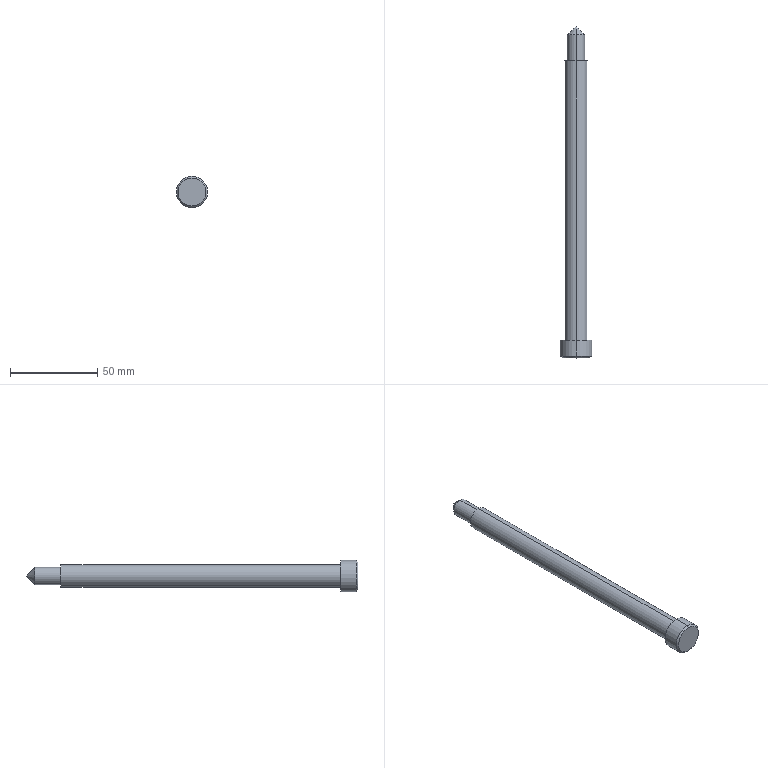Part | STEP file | 1 solid | 13 faces | box 18 x 190 x 18 mm | volume 25064 mm3 | cylinder 6 | cone 4 | plane 3 | commonest cylinder face diameters 10 x2 13 x2 18 x2
STEP:
#1=CARTESIAN_POINT('',(0.,0.,0.));
#2=DIRECTION('',(0.,0.,1.));
#3=DIRECTION('',(1.,0.,0.));
#4=AXIS2_PLACEMENT_3D('',#1,#2,#3);
#5=CARTESIAN_POINT('',(-72.862,-218.5,40.53));
#6=VERTEX_POINT('',#5);
#7=CARTESIAN_POINT('',(-72.862,-218.5,56.53));
#8=VERTEX_POINT('',#7);
#9=CARTESIAN_POINT('',(-72.862,-218.5,48.53));
#10=DIRECTION('',(0.,-1.,0.));
#11=DIRECTION('',(0.,0.,1.));
#12=AXIS2_PLACEMENT_3D('',#9,#10,#11);
#13=CIRCLE('',#12,8.);
#14=CARTESIAN_POINT('',(-72.862,-217.5,48.53));
#15=DIRECTION('',(0.,1.,0.));
#16=DIRECTION('',(0.,0.,1.));
#17=AXIS2_PLACEMENT_3D('',#14,#15,#16);
#18=CONICAL_SURFACE('',#17,9.,0.7854);
#19=CARTESIAN_POINT('',(6.283,-1.));
#20=DIRECTION('',(-1.,0.));
#21=VECTOR('',#20,1.);
#22=LINE('',#19,#21);
#23=(GEOMETRIC_REPRESENTATION_CONTEXT(2)PARAMETRIC_REPRESENTATION_CONTEXT()REPRESENTATION_CONTEXT('',''));
#24=DEFINITIONAL_REPRESENTATION('',(#22),#23);
#25=PCURVE('',#18,#24);
#26=CARTESIAN_POINT('',(-72.862,-218.5,48.53));
#27=DIRECTION('',(0.,1.,0.));
#28=DIRECTION('',(0.,0.,1.));
#29=AXIS2_PLACEMENT_3D('',#26,#27,#28);
#30=PLANE('',#29);
#31=CARTESIAN_POINT('',(8.,0.));
#32=CARTESIAN_POINT('',(8.,-13.856));
#33=CARTESIAN_POINT('',(-4.,-6.928));
#34=CARTESIAN_POINT('',(-16.,0.));
#35=CARTESIAN_POINT('',(-4.,6.928));
#36=CARTESIAN_POINT('',(8.,13.856));
#37=CARTESIAN_POINT('',(8.,0.));
#38=(BOUNDED_CURVE()B_SPLINE_CURVE(2,(#31,#32,#33,#34,#35,#36,#37),.UNSPECIFIED.,.T.,.F.)B_SPLINE_CURVE_WITH_KNOTS((1,2,2,2,2,1),(-2.094,0.,2.094,4.189,6.283,8.378),.UNSPECIFIED.)CURVE()GEOMETRIC_REPRESENTATION_ITEM()RATIONAL_B_SPLINE_CURVE((1.,0.5,1.,0.5,1.,0.5,1.))REPRESENTATION_ITEM(''));
#39=(GEOMETRIC_REPRESENTATION_CONTEXT(2)PARAMETRIC_REPRESENTATION_CONTEXT()REPRESENTATION_CONTEXT('',''));
#40=DEFINITIONAL_REPRESENTATION('',(#38),#39);
#41=PCURVE('',#30,#40);
#42=SURFACE_CURVE('',#13,(#25,#41),.PCURVE_S1.);
#43=EDGE_CURVE('',#6,#8,#42,.T.);
#44=ORIENTED_EDGE('',*,*,#43,.F.);
#45=CARTESIAN_POINT('',(-72.862,-217.5,39.53));
#46=VERTEX_POINT('',#45);
#47=CARTESIAN_POINT('',(-72.862,-217.5,39.53));
#48=DIRECTION('',(0.,0.7071,-0.7071));
#49=VECTOR('',#48,1.);
#50=LINE('',#47,#49);
#51=CARTESIAN_POINT('',(3.142,0.));
#52=DIRECTION('',(0.,1.));
#53=VECTOR('',#52,1.);
#54=LINE('',#51,#53);
#55=(GEOMETRIC_REPRESENTATION_CONTEXT(2)PARAMETRIC_REPRESENTATION_CONTEXT()REPRESENTATION_CONTEXT('',''));
#56=DEFINITIONAL_REPRESENTATION('',(#54),#55);
#57=PCURVE('',#18,#56);
#58=CARTESIAN_POINT('',(-72.862,-217.5,48.53));
#59=DIRECTION('',(0.,1.,0.));
#60=DIRECTION('',(0.,0.,1.));
#61=AXIS2_PLACEMENT_3D('',#58,#59,#60);
#62=CONICAL_SURFACE('',#61,9.,0.7854);
#63=CARTESIAN_POINT('',(3.142,0.));
#64=DIRECTION('',(0.,1.));
#65=VECTOR('',#64,1.);
#66=LINE('',#63,#65);
#67=(GEOMETRIC_REPRESENTATION_CONTEXT(2)PARAMETRIC_REPRESENTATION_CONTEXT()REPRESENTATION_CONTEXT('',''));
#68=DEFINITIONAL_REPRESENTATION('',(#66),#67);
#69=PCURVE('',#62,#68);
#70=SURFACE_CURVE('',#50,(#57,#69),.PCURVE_S1.);
#71=EDGE_CURVE('',#6,#46,#70,.T.);
#72=ORIENTED_EDGE('',*,*,#71,.T.);
#73=CARTESIAN_POINT('',(-72.862,-217.5,57.53));
#74=VERTEX_POINT('',#73);
#75=CARTESIAN_POINT('',(-72.862,-217.5,48.53));
#76=DIRECTION('',(0.,1.,0.));
#77=DIRECTION('',(0.,0.,1.));
#78=AXIS2_PLACEMENT_3D('',#75,#76,#77);
#79=CIRCLE('',#78,9.);
#80=CARTESIAN_POINT('',(0.,0.));
#81=DIRECTION('',(1.,0.));
#82=VECTOR('',#81,1.);
#83=LINE('',#80,#82);
#84=(GEOMETRIC_REPRESENTATION_CONTEXT(2)PARAMETRIC_REPRESENTATION_CONTEXT()REPRESENTATION_CONTEXT('',''));
#85=DEFINITIONAL_REPRESENTATION('',(#83),#84);
#86=PCURVE('',#18,#85);
#87=CARTESIAN_POINT('',(-72.862,-220.,48.53));
#88=DIRECTION('',(0.,1.,0.));
#89=DIRECTION('',(0.,0.,1.));
#90=AXIS2_PLACEMENT_3D('',#87,#88,#89);
#91=CYLINDRICAL_SURFACE('',#90,9.);
#92=CARTESIAN_POINT('',(0.,2.5));
#93=DIRECTION('',(1.,0.));
#94=VECTOR('',#93,1.);
#95=LINE('',#92,#94);
#96=(GEOMETRIC_REPRESENTATION_CONTEXT(2)PARAMETRIC_REPRESENTATION_CONTEXT()REPRESENTATION_CONTEXT('',''));
#97=DEFINITIONAL_REPRESENTATION('',(#95),#96);
#98=PCURVE('',#91,#97);
#99=SURFACE_CURVE('',#79,(#86,#98),.PCURVE_S1.);
#100=EDGE_CURVE('',#74,#46,#99,.T.);
#101=ORIENTED_EDGE('',*,*,#100,.F.);
#102=CARTESIAN_POINT('',(-72.862,-217.5,57.53));
#103=DIRECTION('',(0.,0.7071,0.7071));
#104=VECTOR('',#103,1.);
#105=LINE('',#102,#104);
#106=CARTESIAN_POINT('',(0.,0.));
#107=DIRECTION('',(0.,1.));
#108=VECTOR('',#107,1.);
#109=LINE('',#106,#108);
#110=(GEOMETRIC_REPRESENTATION_CONTEXT(2)PARAMETRIC_REPRESENTATION_CONTEXT()REPRESENTATION_CONTEXT('',''));
#111=DEFINITIONAL_REPRESENTATION('',(#109),#110);
#112=PCURVE('',#18,#111);
#113=CARTESIAN_POINT('',(6.283,0.));
#114=DIRECTION('',(0.,1.));
#115=VECTOR('',#114,1.);
#116=LINE('',#113,#115);
#117=(GEOMETRIC_REPRESENTATION_CONTEXT(2)PARAMETRIC_REPRESENTATION_CONTEXT()REPRESENTATION_CONTEXT('',''));
#118=DEFINITIONAL_REPRESENTATION('',(#116),#117);
#119=PCURVE('',#62,#118);
#120=SURFACE_CURVE('',#105,(#112,#119),.PCURVE_S1.);
#121=EDGE_CURVE('',#8,#74,#120,.T.);
#122=ORIENTED_EDGE('',*,*,#121,.F.);
#123=EDGE_LOOP('',(#44,#72,#101,#122));
#124=FACE_BOUND('',#123,.T.);
#125=ADVANCED_FACE('',(#124),#18,.T.);
#126=CARTESIAN_POINT('',(-72.862,-28.5,48.53));
#127=VERTEX_POINT('',#126);
#128=CARTESIAN_POINT('',(-72.862,-33.5,43.53));
#129=VERTEX_POINT('',#128);
#130=CARTESIAN_POINT('',(-72.862,-33.5,43.53));
#131=DIRECTION('',(0.,-0.7071,-0.7071));
#132=VECTOR('',#131,1.);
#133=LINE('',#130,#132);
#134=CARTESIAN_POINT('',(-72.862,-33.5,48.53));
#135=DIRECTION('',(0.,-1.,0.));
#136=DIRECTION('',(0.,0.,-1.));
#137=AXIS2_PLACEMENT_3D('',#134,#135,#136);
#138=CONICAL_SURFACE('',#137,5.,0.7854);
#139=CARTESIAN_POINT('',(0.,0.));
#140=DIRECTION('',(0.,1.));
#141=VECTOR('',#140,1.);
#142=LINE('',#139,#141);
#143=(GEOMETRIC_REPRESENTATION_CONTEXT(2)PARAMETRIC_REPRESENTATION_CONTEXT()REPRESENTATION_CONTEXT('',''));
#144=DEFINITIONAL_REPRESENTATION('',(#142),#143);
#145=PCURVE('',#138,#144);
#146=CARTESIAN_POINT('',(-72.862,-33.5,48.53));
#147=DIRECTION('',(0.,-1.,0.));
#148=DIRECTION('',(0.,0.,-1.));
#149=AXIS2_PLACEMENT_3D('',#146,#147,#148);
#150=CONICAL_SURFACE('',#149,5.,0.7854);
#151=CARTESIAN_POINT('',(6.283,0.));
#152=DIRECTION('',(0.,1.));
#153=VECTOR('',#152,1.);
#154=LINE('',#151,#153);
#155=(GEOMETRIC_REPRESENTATION_CONTEXT(2)PARAMETRIC_REPRESENTATION_CONTEXT()REPRESENTATION_CONTEXT('',''));
#156=DEFINITIONAL_REPRESENTATION('',(#154),#155);
#157=PCURVE('',#150,#156);
#158=SURFACE_CURVE('',#133,(#145,#157),.PCURVE_S1.);
#159=EDGE_CURVE('',#127,#129,#158,.T.);
#160=ORIENTED_EDGE('',*,*,#159,.F.);
#161=CARTESIAN_POINT('',(-72.862,-33.5,53.53));
#162=VERTEX_POINT('',#161);
#163=CARTESIAN_POINT('',(-72.862,-33.5,53.53));
#164=DIRECTION('',(0.,-0.7071,0.7071));
#165=VECTOR('',#164,1.);
#166=LINE('',#163,#165);
#167=CARTESIAN_POINT('',(3.142,-5.));
#168=CARTESIAN_POINT('',(3.142,-4.924));
#169=CARTESIAN_POINT('',(3.142,-4.773));
#170=CARTESIAN_POINT('',(3.142,-4.545));
#171=CARTESIAN_POINT('',(3.142,-4.318));
#172=CARTESIAN_POINT('',(3.142,-4.091));
#173=CARTESIAN_POINT('',(3.142,-3.864));
#174=CARTESIAN_POINT('',(3.142,-3.636));
#175=CARTESIAN_POINT('',(3.142,-3.409));
#176=CARTESIAN_POINT('',(3.142,-3.182));
#177=CARTESIAN_POINT('',(3.142,-2.955));
#178=CARTESIAN_POINT('',(3.142,-2.727));
#179=CARTESIAN_POINT('',(3.142,-2.5));
#180=CARTESIAN_POINT('',(3.142,-2.273));
#181=CARTESIAN_POINT('',(3.142,-2.045));
#182=CARTESIAN_POINT('',(3.142,-1.818));
#183=CARTESIAN_POINT('',(3.142,-1.591));
#184=CARTESIAN_POINT('',(3.142,-1.364));
#185=CARTESIAN_POINT('',(3.142,-1.136));
#186=CARTESIAN_POINT('',(3.142,-0.9091));
#187=CARTESIAN_POINT('',(3.142,-0.6818));
#188=CARTESIAN_POINT('',(3.142,-0.4545));
#189=CARTESIAN_POINT('',(3.142,-0.2273));
#190=CARTESIAN_POINT('',(3.142,-0.07576));
#191=CARTESIAN_POINT('',(3.142,0.));
#192=B_SPLINE_CURVE_WITH_KNOTS('',3,(#167,#168,#169,#170,#171,#172,#173,#174,#175,#176,#177,#178,#179,#180,#181,#182,#183,#184,#185,#186,#187,#188,#189,#190,#191),.UNSPECIFIED.,.F.,.F.,(4,1,1,1,1,1,1,1,1,1,1,1,1,1,1,1,1,1,1,1,1,1,4),(-7.071,-6.75,-6.428,-6.107,-5.785,-5.464,-5.143,-4.821,-4.5,-4.178,-3.857,-3.536,-3.214,-2.893,-2.571,-2.25,-1.928,-1.607,-1.286,-0.9642,-0.6428,-0.3214,0.),.QUASI_UNIFORM_KNOTS.);
#193=(GEOMETRIC_REPRESENTATION_CONTEXT(2)PARAMETRIC_REPRESENTATION_CONTEXT()REPRESENTATION_CONTEXT('',''));
#194=DEFINITIONAL_REPRESENTATION('',(#192),#193);
#195=PCURVE('',#138,#194);
#196=CARTESIAN_POINT('',(3.142,-5.));
#197=CARTESIAN_POINT('',(3.142,-4.924));
#198=CARTESIAN_POINT('',(3.142,-4.773));
#199=CARTESIAN_POINT('',(3.142,-4.545));
#200=CARTESIAN_POINT('',(3.142,-4.318));
#201=CARTESIAN_POINT('',(3.142,-4.091));
#202=CARTESIAN_POINT('',(3.142,-3.864));
#203=CARTESIAN_POINT('',(3.142,-3.636));
#204=CARTESIAN_POINT('',(3.142,-3.409));
#205=CARTESIAN_POINT('',(3.142,-3.182));
#206=CARTESIAN_POINT('',(3.142,-2.955));
#207=CARTESIAN_POINT('',(3.142,-2.727));
#208=CARTESIAN_POINT('',(3.142,-2.5));
#209=CARTESIAN_POINT('',(3.142,-2.273));
#210=CARTESIAN_POINT('',(3.142,-2.045));
#211=CARTESIAN_POINT('',(3.142,-1.818));
#212=CARTESIAN_POINT('',(3.142,-1.591));
#213=CARTESIAN_POINT('',(3.142,-1.364));
#214=CARTESIAN_POINT('',(3.142,-1.136));
#215=CARTESIAN_POINT('',(3.142,-0.9091));
#216=CARTESIAN_POINT('',(3.142,-0.6818));
#217=CARTESIAN_POINT('',(3.142,-0.4545));
#218=CARTESIAN_POINT('',(3.142,-0.2273));
#219=CARTESIAN_POINT('',(3.142,-0.07576));
#220=CARTESIAN_POINT('',(3.142,0.));
#221=B_SPLINE_CURVE_WITH_KNOTS('',3,(#196,#197,#198,#199,#200,#201,#202,#203,#204,#205,#206,#207,#208,#209,#210,#211,#212,#213,#214,#215,#216,#217,#218,#219,#220),.UNSPECIFIED.,.F.,.F.,(4,1,1,1,1,1,1,1,1,1,1,1,1,1,1,1,1,1,1,1,1,1,4),(-7.071,-6.75,-6.428,-6.107,-5.785,-5.464,-5.143,-4.821,-4.5,-4.178,-3.857,-3.536,-3.214,-2.893,-2.571,-2.25,-1.928,-1.607,-1.286,-0.9642,-0.6428,-0.3214,0.),.QUASI_UNIFORM_KNOTS.);
#222=(GEOMETRIC_REPRESENTATION_CONTEXT(2)PARAMETRIC_REPRESENTATION_CONTEXT()REPRESENTATION_CONTEXT('',''));
#223=DEFINITIONAL_REPRESENTATION('',(#221),#222);
#224=PCURVE('',#150,#223);
#225=SURFACE_CURVE('',#166,(#195,#224),.PCURVE_S1.);
#226=EDGE_CURVE('',#127,#162,#225,.T.);
#227=ORIENTED_EDGE('',*,*,#226,.T.);
#228=CARTESIAN_POINT('',(-72.862,-33.5,48.53));
#229=DIRECTION('',(0.,-1.,0.));
#230=DIRECTION('',(0.,0.,1.));
#231=AXIS2_PLACEMENT_3D('',#228,#229,#230);
#232=CIRCLE('',#231,5.);
#233=CARTESIAN_POINT('',(-3.142,0.));
#234=DIRECTION('',(1.,0.));
#235=VECTOR('',#234,1.);
#236=LINE('',#233,#235);
#237=(GEOMETRIC_REPRESENTATION_CONTEXT(2)PARAMETRIC_REPRESENTATION_CONTEXT()REPRESENTATION_CONTEXT('',''));
#238=DEFINITIONAL_REPRESENTATION('',(#236),#237);
#239=PCURVE('',#138,#238);
#240=CARTESIAN_POINT('',(-72.862,-48.5,48.53));
#241=DIRECTION('',(0.,1.,0.));
#242=DIRECTION('',(0.,0.,1.));
#243=AXIS2_PLACEMENT_3D('',#240,#241,#242);
#244=CYLINDRICAL_SURFACE('',#243,5.);
#245=CARTESIAN_POINT('',(6.283,15.));
#246=DIRECTION('',(-1.,0.));
#247=VECTOR('',#246,1.);
#248=LINE('',#245,#247);
#249=(GEOMETRIC_REPRESENTATION_CONTEXT(2)PARAMETRIC_REPRESENTATION_CONTEXT()REPRESENTATION_CONTEXT('',''));
#250=DEFINITIONAL_REPRESENTATION('',(#248),#249);
#251=PCURVE('',#244,#250);
#252=SURFACE_CURVE('',#232,(#239,#251),.PCURVE_S1.);
#253=EDGE_CURVE('',#129,#162,#252,.T.);
#254=ORIENTED_EDGE('',*,*,#253,.F.);
#255=EDGE_LOOP('',(#160,#227,#254));
#256=FACE_BOUND('',#255,.T.);
#257=ADVANCED_FACE('',(#256),#138,.T.);
#258=CARTESIAN_POINT('',(-72.862,-48.5,53.53));
#259=VERTEX_POINT('',#258);
#260=CARTESIAN_POINT('',(-72.862,-48.5,43.53));
#261=VERTEX_POINT('',#260);
#262=CARTESIAN_POINT('',(-72.862,-48.5,48.53));
#263=DIRECTION('',(0.,1.,0.));
#264=DIRECTION('',(0.,0.,1.));
#265=AXIS2_PLACEMENT_3D('',#262,#263,#264);
#266=CIRCLE('',#265,5.);
#267=CARTESIAN_POINT('',(0.,0.));
#268=DIRECTION('',(1.,0.));
#269=VECTOR('',#268,1.);
#270=LINE('',#267,#269);
#271=(GEOMETRIC_REPRESENTATION_CONTEXT(2)PARAMETRIC_REPRESENTATION_CONTEXT()REPRESENTATION_CONTEXT('',''));
#272=DEFINITIONAL_REPRESENTATION('',(#270),#271);
#273=PCURVE('',#244,#272);
#274=CARTESIAN_POINT('',(-72.862,-48.5,48.53));
#275=DIRECTION('',(0.,1.,0.));
#276=DIRECTION('',(0.,0.,1.));
#277=AXIS2_PLACEMENT_3D('',#274,#275,#276);
#278=PLANE('',#277);
#279=CARTESIAN_POINT('',(0.,0.));
#280=DIRECTION('',(1.,0.));
#281=AXIS2_PLACEMENT_2D('',#279,#280);
#282=CIRCLE('',#281,5.);
#283=(GEOMETRIC_REPRESENTATION_CONTEXT(2)PARAMETRIC_REPRESENTATION_CONTEXT()REPRESENTATION_CONTEXT('',''));
#284=DEFINITIONAL_REPRESENTATION('',(#282),#283);
#285=PCURVE('',#278,#284);
#286=SURFACE_CURVE('',#266,(#273,#285),.PCURVE_S1.);
#287=EDGE_CURVE('',#259,#261,#286,.T.);
#288=ORIENTED_EDGE('',*,*,#287,.T.);
#289=CARTESIAN_POINT('',(-72.862,-48.5,43.53));
#290=DIRECTION('',(0.,1.,0.));
#291=VECTOR('',#290,1.);
#292=LINE('',#289,#291);
#293=CARTESIAN_POINT('',(3.142,0.));
#294=DIRECTION('',(0.,1.));
#295=VECTOR('',#294,1.);
#296=LINE('',#293,#295);
#297=(GEOMETRIC_REPRESENTATION_CONTEXT(2)PARAMETRIC_REPRESENTATION_CONTEXT()REPRESENTATION_CONTEXT('',''));
#298=DEFINITIONAL_REPRESENTATION('',(#296),#297);
#299=PCURVE('',#244,#298);
#300=CARTESIAN_POINT('',(-72.862,-48.5,48.53));
#301=DIRECTION('',(0.,1.,0.));
#302=DIRECTION('',(0.,0.,1.));
#303=AXIS2_PLACEMENT_3D('',#300,#301,#302);
#304=CYLINDRICAL_SURFACE('',#303,5.);
#305=CARTESIAN_POINT('',(3.142,0.));
#306=DIRECTION('',(0.,1.));
#307=VECTOR('',#306,1.);
#308=LINE('',#305,#307);
#309=(GEOMETRIC_REPRESENTATION_CONTEXT(2)PARAMETRIC_REPRESENTATION_CONTEXT()REPRESENTATION_CONTEXT('',''));
#310=DEFINITIONAL_REPRESENTATION('',(#308),#309);
#311=PCURVE('',#304,#310);
#312=SURFACE_CURVE('',#292,(#299,#311),.PCURVE_S1.);
#313=EDGE_CURVE('',#261,#129,#312,.T.);
#314=ORIENTED_EDGE('',*,*,#313,.T.);
#315=ORIENTED_EDGE('',*,*,#253,.T.);
#316=CARTESIAN_POINT('',(-72.862,-48.5,53.53));
#317=DIRECTION('',(0.,1.,0.));
#318=VECTOR('',#317,1.);
#319=LINE('',#316,#318);
#320=CARTESIAN_POINT('',(0.,0.));
#321=DIRECTION('',(0.,1.));
#322=VECTOR('',#321,1.);
#323=LINE('',#320,#322);
#324=(GEOMETRIC_REPRESENTATION_CONTEXT(2)PARAMETRIC_REPRESENTATION_CONTEXT()REPRESENTATION_CONTEXT('',''));
#325=DEFINITIONAL_REPRESENTATION('',(#323),#324);
#326=PCURVE('',#244,#325);
#327=CARTESIAN_POINT('',(6.283,0.));
#328=DIRECTION('',(0.,1.));
#329=VECTOR('',#328,1.);
#330=LINE('',#327,#329);
#331=(GEOMETRIC_REPRESENTATION_CONTEXT(2)PARAMETRIC_REPRESENTATION_CONTEXT()REPRESENTATION_CONTEXT('',''));
#332=DEFINITIONAL_REPRESENTATION('',(#330),#331);
#333=PCURVE('',#304,#332);
#334=SURFACE_CURVE('',#319,(#326,#333),.PCURVE_S1.);
#335=EDGE_CURVE('',#259,#162,#334,.T.);
#336=ORIENTED_EDGE('',*,*,#335,.F.);
#337=EDGE_LOOP('',(#288,#314,#315,#336));
#338=FACE_BOUND('',#337,.T.);
#339=ADVANCED_FACE('',(#338),#244,.T.);
#340=CARTESIAN_POINT('',(-72.862,-208.5,55.03));
#341=VERTEX_POINT('',#340);
#342=CARTESIAN_POINT('',(-72.862,-208.5,42.03));
#343=VERTEX_POINT('',#342);
#344=CARTESIAN_POINT('',(-72.862,-208.5,48.53));
#345=DIRECTION('',(0.,1.,0.));
#346=DIRECTION('',(0.,0.,-1.));
#347=AXIS2_PLACEMENT_3D('',#344,#345,#346);
#348=CIRCLE('',#347,6.5);
#349=CARTESIAN_POINT('',(-72.862,-220.,48.53));
#350=DIRECTION('',(0.,1.,0.));
#351=DIRECTION('',(0.,0.,1.));
#352=AXIS2_PLACEMENT_3D('',#349,#350,#351);
#353=CYLINDRICAL_SURFACE('',#352,6.5);
#354=CARTESIAN_POINT('',(-3.142,11.5));
#355=DIRECTION('',(1.,0.));
#356=VECTOR('',#355,1.);
#357=LINE('',#354,#356);
#358=(GEOMETRIC_REPRESENTATION_CONTEXT(2)PARAMETRIC_REPRESENTATION_CONTEXT()REPRESENTATION_CONTEXT('',''));
#359=DEFINITIONAL_REPRESENTATION('',(#357),#358);
#360=PCURVE('',#353,#359);
#361=CARTESIAN_POINT('',(-72.862,-208.5,48.53));
#362=DIRECTION('',(0.,-1.,0.));
#363=DIRECTION('',(0.,0.,-1.));
#364=AXIS2_PLACEMENT_3D('',#361,#362,#363);
#365=PLANE('',#364);
#366=CARTESIAN_POINT('',(6.5,0.));
#367=CARTESIAN_POINT('',(6.5,-11.258));
#368=CARTESIAN_POINT('',(-3.25,-5.629));
#369=CARTESIAN_POINT('',(-13.,0.));
#370=CARTESIAN_POINT('',(-3.25,5.629));
#371=CARTESIAN_POINT('',(6.5,11.258));
#372=CARTESIAN_POINT('',(6.5,0.));
#373=(BOUNDED_CURVE()B_SPLINE_CURVE(2,(#366,#367,#368,#369,#370,#371,#372),.UNSPECIFIED.,.T.,.F.)B_SPLINE_CURVE_WITH_KNOTS((1,2,2,2,2,1),(-2.094,0.,2.094,4.189,6.283,8.378),.UNSPECIFIED.)CURVE()GEOMETRIC_REPRESENTATION_ITEM()RATIONAL_B_SPLINE_CURVE((1.,0.5,1.,0.5,1.,0.5,1.))REPRESENTATION_ITEM(''));
#374=(GEOMETRIC_REPRESENTATION_CONTEXT(2)PARAMETRIC_REPRESENTATION_CONTEXT()REPRESENTATION_CONTEXT('',''));
#375=DEFINITIONAL_REPRESENTATION('',(#373),#374);
#376=PCURVE('',#365,#375);
#377=SURFACE_CURVE('',#348,(#360,#376),.PCURVE_S1.);
#378=EDGE_CURVE('',#341,#343,#377,.T.);
#379=ORIENTED_EDGE('',*,*,#378,.T.);
#380=CARTESIAN_POINT('',(-72.862,-48.5,42.03));
#381=VERTEX_POINT('',#380);
#382=CARTESIAN_POINT('',(-72.862,-220.,42.03));
#383=DIRECTION('',(0.,1.,0.));
#384=VECTOR('',#383,1.);
#385=LINE('',#382,#384);
#386=CARTESIAN_POINT('',(3.142,0.));
#387=DIRECTION('',(0.,1.));
#388=VECTOR('',#387,1.);
#389=LINE('',#386,#388);
#390=(GEOMETRIC_REPRESENTATION_CONTEXT(2)PARAMETRIC_REPRESENTATION_CONTEXT()REPRESENTATION_CONTEXT('',''));
#391=DEFINITIONAL_REPRESENTATION('',(#389),#390);
#392=PCURVE('',#353,#391);
#393=CARTESIAN_POINT('',(-72.862,-220.,48.53));
#394=DIRECTION('',(0.,1.,0.));
#395=DIRECTION('',(0.,0.,1.));
#396=AXIS2_PLACEMENT_3D('',#393,#394,#395);
#397=CYLINDRICAL_SURFACE('',#396,6.5);
#398=CARTESIAN_POINT('',(3.142,0.));
#399=DIRECTION('',(0.,1.));
#400=VECTOR('',#399,1.);
#401=LINE('',#398,#400);
#402=(GEOMETRIC_REPRESENTATION_CONTEXT(2)PARAMETRIC_REPRESENTATION_CONTEXT()REPRESENTATION_CONTEXT('',''));
#403=DEFINITIONAL_REPRESENTATION('',(#401),#402);
#404=PCURVE('',#397,#403);
#405=SURFACE_CURVE('',#385,(#392,#404),.PCURVE_S1.);
#406=EDGE_CURVE('',#343,#381,#405,.T.);
#407=ORIENTED_EDGE('',*,*,#406,.T.);
#408=CARTESIAN_POINT('',(-72.862,-48.5,55.03));
#409=VERTEX_POINT('',#408);
#410=CARTESIAN_POINT('',(-72.862,-48.5,48.53));
#411=DIRECTION('',(0.,1.,0.));
#412=DIRECTION('',(0.,0.,1.));
#413=AXIS2_PLACEMENT_3D('',#410,#411,#412);
#414=CIRCLE('',#413,6.5);
#415=CARTESIAN_POINT('',(0.,171.5));
#416=DIRECTION('',(1.,0.));
#417=VECTOR('',#416,1.);
#418=LINE('',#415,#417);
#419=(GEOMETRIC_REPRESENTATION_CONTEXT(2)PARAMETRIC_REPRESENTATION_CONTEXT()REPRESENTATION_CONTEXT('',''));
#420=DEFINITIONAL_REPRESENTATION('',(#418),#419);
#421=PCURVE('',#353,#420);
#422=CARTESIAN_POINT('',(0.,0.));
#423=DIRECTION('',(1.,0.));
#424=AXIS2_PLACEMENT_2D('',#422,#423);
#425=CIRCLE('',#424,6.5);
#426=(GEOMETRIC_REPRESENTATION_CONTEXT(2)PARAMETRIC_REPRESENTATION_CONTEXT()REPRESENTATION_CONTEXT('',''));
#427=DEFINITIONAL_REPRESENTATION('',(#425),#426);
#428=PCURVE('',#278,#427);
#429=SURFACE_CURVE('',#414,(#421,#428),.PCURVE_S1.);
#430=EDGE_CURVE('',#409,#381,#429,.T.);
#431=ORIENTED_EDGE('',*,*,#430,.F.);
#432=CARTESIAN_POINT('',(-72.862,-220.,55.03));
#433=DIRECTION('',(0.,1.,0.));
#434=VECTOR('',#433,1.);
#435=LINE('',#432,#434);
#436=CARTESIAN_POINT('',(0.,0.));
#437=DIRECTION('',(0.,1.));
#438=VECTOR('',#437,1.);
#439=LINE('',#436,#438);
#440=(GEOMETRIC_REPRESENTATION_CONTEXT(2)PARAMETRIC_REPRESENTATION_CONTEXT()REPRESENTATION_CONTEXT('',''));
#441=DEFINITIONAL_REPRESENTATION('',(#439),#440);
#442=PCURVE('',#353,#441);
#443=CARTESIAN_POINT('',(6.283,0.));
#444=DIRECTION('',(0.,1.));
#445=VECTOR('',#444,1.);
#446=LINE('',#443,#445);
#447=(GEOMETRIC_REPRESENTATION_CONTEXT(2)PARAMETRIC_REPRESENTATION_CONTEXT()REPRESENTATION_CONTEXT('',''));
#448=DEFINITIONAL_REPRESENTATION('',(#446),#447);
#449=PCURVE('',#397,#448);
#450=SURFACE_CURVE('',#435,(#442,#449),.PCURVE_S1.);
#451=EDGE_CURVE('',#341,#409,#450,.T.);
#452=ORIENTED_EDGE('',*,*,#451,.F.);
#453=EDGE_LOOP('',(#379,#407,#431,#452));
#454=FACE_BOUND('',#453,.T.);
#455=ADVANCED_FACE('',(#454),#353,.T.);
#456=ORIENTED_EDGE('',*,*,#100,.T.);
#457=CARTESIAN_POINT('',(-72.862,-208.5,39.53));
#458=VERTEX_POINT('',#457);
#459=CARTESIAN_POINT('',(-72.862,-220.,39.53));
#460=DIRECTION('',(0.,1.,0.));
#461=VECTOR('',#460,1.);
#462=LINE('',#459,#461);
#463=CARTESIAN_POINT('',(3.142,0.));
#464=DIRECTION('',(0.,1.));
#465=VECTOR('',#464,1.);
#466=LINE('',#463,#465);
#467=(GEOMETRIC_REPRESENTATION_CONTEXT(2)PARAMETRIC_REPRESENTATION_CONTEXT()REPRESENTATION_CONTEXT('',''));
#468=DEFINITIONAL_REPRESENTATION('',(#466),#467);
#469=PCURVE('',#91,#468);
#470=CARTESIAN_POINT('',(-72.862,-220.,48.53));
#471=DIRECTION('',(0.,1.,0.));
#472=DIRECTION('',(0.,0.,1.));
#473=AXIS2_PLACEMENT_3D('',#470,#471,#472);
#474=CYLINDRICAL_SURFACE('',#473,9.);
#475=CARTESIAN_POINT('',(3.142,0.));
#476=DIRECTION('',(0.,1.));
#477=VECTOR('',#476,1.);
#478=LINE('',#475,#477);
#479=(GEOMETRIC_REPRESENTATION_CONTEXT(2)PARAMETRIC_REPRESENTATION_CONTEXT()REPRESENTATION_CONTEXT('',''));
#480=DEFINITIONAL_REPRESENTATION('',(#478),#479);
#481=PCURVE('',#474,#480);
#482=SURFACE_CURVE('',#462,(#469,#481),.PCURVE_S1.);
#483=EDGE_CURVE('',#46,#458,#482,.T.);
#484=ORIENTED_EDGE('',*,*,#483,.T.);
#485=CARTESIAN_POINT('',(-72.862,-208.5,57.53));
#486=VERTEX_POINT('',#485);
#487=CARTESIAN_POINT('',(-72.862,-208.5,48.53));
#488=DIRECTION('',(0.,1.,0.));
#489=DIRECTION('',(0.,0.,-1.));
#490=AXIS2_PLACEMENT_3D('',#487,#488,#489);
#491=CIRCLE('',#490,9.);
#492=CARTESIAN_POINT('',(-3.142,11.5));
#493=DIRECTION('',(1.,0.));
#494=VECTOR('',#493,1.);
#495=LINE('',#492,#494);
#496=(GEOMETRIC_REPRESENTATION_CONTEXT(2)PARAMETRIC_REPRESENTATION_CONTEXT()REPRESENTATION_CONTEXT('',''));
#497=DEFINITIONAL_REPRESENTATION('',(#495),#496);
#498=PCURVE('',#91,#497);
#499=CARTESIAN_POINT('',(9.,0.));
#500=CARTESIAN_POINT('',(9.,-15.588));
#501=CARTESIAN_POINT('',(-4.5,-7.794));
#502=CARTESIAN_POINT('',(-18.,0.));
#503=CARTESIAN_POINT('',(-4.5,7.794));
#504=CARTESIAN_POINT('',(9.,15.588));
#505=CARTESIAN_POINT('',(9.,0.));
#506=(BOUNDED_CURVE()B_SPLINE_CURVE(2,(#499,#500,#501,#502,#503,#504,#505),.UNSPECIFIED.,.T.,.F.)B_SPLINE_CURVE_WITH_KNOTS((1,2,2,2,2,1),(-2.094,0.,2.094,4.189,6.283,8.378),.UNSPECIFIED.)CURVE()GEOMETRIC_REPRESENTATION_ITEM()RATIONAL_B_SPLINE_CURVE((1.,0.5,1.,0.5,1.,0.5,1.))REPRESENTATION_ITEM(''));
#507=(GEOMETRIC_REPRESENTATION_CONTEXT(2)PARAMETRIC_REPRESENTATION_CONTEXT()REPRESENTATION_CONTEXT('',''));
#508=DEFINITIONAL_REPRESENTATION('',(#506),#507);
#509=PCURVE('',#365,#508);
#510=SURFACE_CURVE('',#491,(#498,#509),.PCURVE_S1.);
#511=EDGE_CURVE('',#486,#458,#510,.T.);
#512=ORIENTED_EDGE('',*,*,#511,.F.);
#513=CARTESIAN_POINT('',(-72.862,-220.,57.53));
#514=DIRECTION('',(0.,1.,0.));
#515=VECTOR('',#514,1.);
#516=LINE('',#513,#515);
#517=CARTESIAN_POINT('',(0.,0.));
#518=DIRECTION('',(0.,1.));
#519=VECTOR('',#518,1.);
#520=LINE('',#517,#519);
#521=(GEOMETRIC_REPRESENTATION_CONTEXT(2)PARAMETRIC_REPRESENTATION_CONTEXT()REPRESENTATION_CONTEXT('',''));
#522=DEFINITIONAL_REPRESENTATION('',(#520),#521);
#523=PCURVE('',#91,#522);
#524=CARTESIAN_POINT('',(6.283,0.));
#525=DIRECTION('',(0.,1.));
#526=VECTOR('',#525,1.);
#527=LINE('',#524,#526);
#528=(GEOMETRIC_REPRESENTATION_CONTEXT(2)PARAMETRIC_REPRESENTATION_CONTEXT()REPRESENTATION_CONTEXT('',''));
#529=DEFINITIONAL_REPRESENTATION('',(#527),#528);
#530=PCURVE('',#474,#529);
#531=SURFACE_CURVE('',#516,(#523,#530),.PCURVE_S1.);
#532=EDGE_CURVE('',#74,#486,#531,.T.);
#533=ORIENTED_EDGE('',*,*,#532,.F.);
#534=EDGE_LOOP('',(#456,#484,#512,#533));
#535=FACE_BOUND('',#534,.T.);
#536=ADVANCED_FACE('',(#535),#91,.T.);
#537=ORIENTED_EDGE('',*,*,#511,.T.);
#538=CARTESIAN_POINT('',(-72.862,-208.5,48.53));
#539=DIRECTION('',(0.,1.,0.));
#540=DIRECTION('',(0.,0.,-1.));
#541=AXIS2_PLACEMENT_3D('',#538,#539,#540);
#542=CIRCLE('',#541,9.);
#543=CARTESIAN_POINT('',(9.,0.));
#544=CARTESIAN_POINT('',(9.,-15.588));
#545=CARTESIAN_POINT('',(-4.5,-7.794));
#546=CARTESIAN_POINT('',(-18.,0.));
#547=CARTESIAN_POINT('',(-4.5,7.794));
#548=CARTESIAN_POINT('',(9.,15.588));
#549=CARTESIAN_POINT('',(9.,0.));
#550=(BOUNDED_CURVE()B_SPLINE_CURVE(2,(#543,#544,#545,#546,#547,#548,#549),.UNSPECIFIED.,.T.,.F.)B_SPLINE_CURVE_WITH_KNOTS((1,2,2,2,2,1),(-2.094,0.,2.094,4.189,6.283,8.378),.UNSPECIFIED.)CURVE()GEOMETRIC_REPRESENTATION_ITEM()RATIONAL_B_SPLINE_CURVE((1.,0.5,1.,0.5,1.,0.5,1.))REPRESENTATION_ITEM(''));
#551=(GEOMETRIC_REPRESENTATION_CONTEXT(2)PARAMETRIC_REPRESENTATION_CONTEXT()REPRESENTATION_CONTEXT('',''));
#552=DEFINITIONAL_REPRESENTATION('',(#550),#551);
#553=PCURVE('',#365,#552);
#554=CARTESIAN_POINT('',(3.142,11.5));
#555=DIRECTION('',(1.,0.));
#556=VECTOR('',#555,1.);
#557=LINE('',#554,#556);
#558=(GEOMETRIC_REPRESENTATION_CONTEXT(2)PARAMETRIC_REPRESENTATION_CONTEXT()REPRESENTATION_CONTEXT('',''));
#559=DEFINITIONAL_REPRESENTATION('',(#557),#558);
#560=PCURVE('',#474,#559);
#561=SURFACE_CURVE('',#542,(#553,#560),.PCURVE_S1.);
#562=EDGE_CURVE('',#458,#486,#561,.T.);
#563=ORIENTED_EDGE('',*,*,#562,.T.);
#564=EDGE_LOOP('',(#537,#563));
#565=FACE_BOUND('',#564,.T.);
#566=ORIENTED_EDGE('',*,*,#378,.F.);
#567=CARTESIAN_POINT('',(-72.862,-208.5,48.53));
#568=DIRECTION('',(0.,1.,0.));
#569=DIRECTION('',(0.,0.,-1.));
#570=AXIS2_PLACEMENT_3D('',#567,#568,#569);
#571=CIRCLE('',#570,6.5);
#572=CARTESIAN_POINT('',(6.5,0.));
#573=CARTESIAN_POINT('',(6.5,-11.258));
#574=CARTESIAN_POINT('',(-3.25,-5.629));
#575=CARTESIAN_POINT('',(-13.,0.));
#576=CARTESIAN_POINT('',(-3.25,5.629));
#577=CARTESIAN_POINT('',(6.5,11.258));
#578=CARTESIAN_POINT('',(6.5,0.));
#579=(BOUNDED_CURVE()B_SPLINE_CURVE(2,(#572,#573,#574,#575,#576,#577,#578),.UNSPECIFIED.,.T.,.F.)B_SPLINE_CURVE_WITH_KNOTS((1,2,2,2,2,1),(-2.094,0.,2.094,4.189,6.283,8.378),.UNSPECIFIED.)CURVE()GEOMETRIC_REPRESENTATION_ITEM()RATIONAL_B_SPLINE_CURVE((1.,0.5,1.,0.5,1.,0.5,1.))REPRESENTATION_ITEM(''));
#580=(GEOMETRIC_REPRESENTATION_CONTEXT(2)PARAMETRIC_REPRESENTATION_CONTEXT()REPRESENTATION_CONTEXT('',''));
#581=DEFINITIONAL_REPRESENTATION('',(#579),#580);
#582=PCURVE('',#365,#581);
#583=CARTESIAN_POINT('',(3.142,11.5));
#584=DIRECTION('',(1.,0.));
#585=VECTOR('',#584,1.);
#586=LINE('',#583,#585);
#587=(GEOMETRIC_REPRESENTATION_CONTEXT(2)PARAMETRIC_REPRESENTATION_CONTEXT()REPRESENTATION_CONTEXT('',''));
#588=DEFINITIONAL_REPRESENTATION('',(#586),#587);
#589=PCURVE('',#397,#588);
#590=SURFACE_CURVE('',#571,(#582,#589),.PCURVE_S1.);
#591=EDGE_CURVE('',#343,#341,#590,.T.);
#592=ORIENTED_EDGE('',*,*,#591,.F.);
#593=EDGE_LOOP('',(#566,#592));
#594=FACE_BOUND('',#593,.T.);
#595=ADVANCED_FACE('',(#565,#594),#365,.F.);
#596=ORIENTED_EDGE('',*,*,#483,.F.);
#597=CARTESIAN_POINT('',(-72.862,-217.5,48.53));
#598=DIRECTION('',(0.,1.,0.));
#599=DIRECTION('',(0.,0.,1.));
#600=AXIS2_PLACEMENT_3D('',#597,#598,#599);
#601=CIRCLE('',#600,9.);
#602=CARTESIAN_POINT('',(0.,2.5));
#603=DIRECTION('',(1.,0.));
#604=VECTOR('',#603,1.);
#605=LINE('',#602,#604);
#606=(GEOMETRIC_REPRESENTATION_CONTEXT(2)PARAMETRIC_REPRESENTATION_CONTEXT()REPRESENTATION_CONTEXT('',''));
#607=DEFINITIONAL_REPRESENTATION('',(#605),#606);
#608=PCURVE('',#474,#607);
#609=CARTESIAN_POINT('',(0.,0.));
#610=DIRECTION('',(1.,0.));
#611=VECTOR('',#610,1.);
#612=LINE('',#609,#611);
#613=(GEOMETRIC_REPRESENTATION_CONTEXT(2)PARAMETRIC_REPRESENTATION_CONTEXT()REPRESENTATION_CONTEXT('',''));
#614=DEFINITIONAL_REPRESENTATION('',(#612),#613);
#615=PCURVE('',#62,#614);
#616=SURFACE_CURVE('',#601,(#608,#615),.PCURVE_S1.);
#617=EDGE_CURVE('',#46,#74,#616,.T.);
#618=ORIENTED_EDGE('',*,*,#617,.T.);
#619=ORIENTED_EDGE('',*,*,#532,.T.);
#620=ORIENTED_EDGE('',*,*,#562,.F.);
#621=EDGE_LOOP('',(#596,#618,#619,#620));
#622=FACE_BOUND('',#621,.T.);
#623=ADVANCED_FACE('',(#622),#474,.T.);
#624=CARTESIAN_POINT('',(-72.862,-218.5,48.53));
#625=DIRECTION('',(0.,-1.,0.));
#626=DIRECTION('',(0.,0.,1.));
#627=AXIS2_PLACEMENT_3D('',#624,#625,#626);
#628=CIRCLE('',#627,8.);
#629=CARTESIAN_POINT('',(8.,0.));
#630=CARTESIAN_POINT('',(8.,-13.856));
#631=CARTESIAN_POINT('',(-4.,-6.928));
#632=CARTESIAN_POINT('',(-16.,0.));
#633=CARTESIAN_POINT('',(-4.,6.928));
#634=CARTESIAN_POINT('',(8.,13.856));
#635=CARTESIAN_POINT('',(8.,0.));
#636=(BOUNDED_CURVE()B_SPLINE_CURVE(2,(#629,#630,#631,#632,#633,#634,#635),.UNSPECIFIED.,.T.,.F.)B_SPLINE_CURVE_WITH_KNOTS((1,2,2,2,2,1),(-2.094,0.,2.094,4.189,6.283,8.378),.UNSPECIFIED.)CURVE()GEOMETRIC_REPRESENTATION_ITEM()RATIONAL_B_SPLINE_CURVE((1.,0.5,1.,0.5,1.,0.5,1.))REPRESENTATION_ITEM(''));
#637=(GEOMETRIC_REPRESENTATION_CONTEXT(2)PARAMETRIC_REPRESENTATION_CONTEXT()REPRESENTATION_CONTEXT('',''));
#638=DEFINITIONAL_REPRESENTATION('',(#636),#637);
#639=PCURVE('',#30,#638);
#640=CARTESIAN_POINT('',(6.283,-1.));
#641=DIRECTION('',(-1.,0.));
#642=VECTOR('',#641,1.);
#643=LINE('',#640,#642);
#644=(GEOMETRIC_REPRESENTATION_CONTEXT(2)PARAMETRIC_REPRESENTATION_CONTEXT()REPRESENTATION_CONTEXT('',''));
#645=DEFINITIONAL_REPRESENTATION('',(#643),#644);
#646=PCURVE('',#62,#645);
#647=SURFACE_CURVE('',#628,(#639,#646),.PCURVE_S1.);
#648=EDGE_CURVE('',#8,#6,#647,.T.);
#649=ORIENTED_EDGE('',*,*,#648,.T.);
#650=ORIENTED_EDGE('',*,*,#43,.T.);
#651=EDGE_LOOP('',(#649,#650));
#652=FACE_BOUND('',#651,.T.);
#653=ADVANCED_FACE('',(#652),#30,.F.);
#654=ORIENTED_EDGE('',*,*,#287,.F.);
#655=CARTESIAN_POINT('',(-72.862,-48.5,48.53));
#656=DIRECTION('',(0.,1.,0.));
#657=DIRECTION('',(0.,0.,1.));
#658=AXIS2_PLACEMENT_3D('',#655,#656,#657);
#659=CIRCLE('',#658,5.);
#660=CARTESIAN_POINT('',(0.,0.));
#661=DIRECTION('',(1.,0.));
#662=AXIS2_PLACEMENT_2D('',#660,#661);
#663=CIRCLE('',#662,5.);
#664=(GEOMETRIC_REPRESENTATION_CONTEXT(2)PARAMETRIC_REPRESENTATION_CONTEXT()REPRESENTATION_CONTEXT('',''));
#665=DEFINITIONAL_REPRESENTATION('',(#663),#664);
#666=PCURVE('',#278,#665);
#667=CARTESIAN_POINT('',(0.,0.));
#668=DIRECTION('',(1.,0.));
#669=VECTOR('',#668,1.);
#670=LINE('',#667,#669);
#671=(GEOMETRIC_REPRESENTATION_CONTEXT(2)PARAMETRIC_REPRESENTATION_CONTEXT()REPRESENTATION_CONTEXT('',''));
#672=DEFINITIONAL_REPRESENTATION('',(#670),#671);
#673=PCURVE('',#304,#672);
#674=SURFACE_CURVE('',#659,(#666,#673),.PCURVE_S1.);
#675=EDGE_CURVE('',#261,#259,#674,.T.);
#676=ORIENTED_EDGE('',*,*,#675,.F.);
#677=EDGE_LOOP('',(#654,#676));
#678=FACE_BOUND('',#677,.T.);
#679=ORIENTED_EDGE('',*,*,#430,.T.);
#680=CARTESIAN_POINT('',(-72.862,-48.5,48.53));
#681=DIRECTION('',(0.,1.,0.));
#682=DIRECTION('',(0.,0.,1.));
#683=AXIS2_PLACEMENT_3D('',#680,#681,#682);
#684=CIRCLE('',#683,6.5);
#685=CARTESIAN_POINT('',(0.,0.));
#686=DIRECTION('',(1.,0.));
#687=AXIS2_PLACEMENT_2D('',#685,#686);
#688=CIRCLE('',#687,6.5);
#689=(GEOMETRIC_REPRESENTATION_CONTEXT(2)PARAMETRIC_REPRESENTATION_CONTEXT()REPRESENTATION_CONTEXT('',''));
#690=DEFINITIONAL_REPRESENTATION('',(#688),#689);
#691=PCURVE('',#278,#690);
#692=CARTESIAN_POINT('',(0.,171.5));
#693=DIRECTION('',(1.,0.));
#694=VECTOR('',#693,1.);
#695=LINE('',#692,#694);
#696=(GEOMETRIC_REPRESENTATION_CONTEXT(2)PARAMETRIC_REPRESENTATION_CONTEXT()REPRESENTATION_CONTEXT('',''));
#697=DEFINITIONAL_REPRESENTATION('',(#695),#696);
#698=PCURVE('',#397,#697);
#699=SURFACE_CURVE('',#684,(#691,#698),.PCURVE_S1.);
#700=EDGE_CURVE('',#381,#409,#699,.T.);
#701=ORIENTED_EDGE('',*,*,#700,.T.);
#702=EDGE_LOOP('',(#679,#701));
#703=FACE_BOUND('',#702,.T.);
#704=ADVANCED_FACE('',(#678,#703),#278,.T.);
#705=ORIENTED_EDGE('',*,*,#406,.F.);
#706=ORIENTED_EDGE('',*,*,#591,.T.);
#707=ORIENTED_EDGE('',*,*,#451,.T.);
#708=ORIENTED_EDGE('',*,*,#700,.F.);
#709=EDGE_LOOP('',(#705,#706,#707,#708));
#710=FACE_BOUND('',#709,.T.);
#711=ADVANCED_FACE('',(#710),#397,.T.);
#712=ORIENTED_EDGE('',*,*,#313,.F.);
#713=ORIENTED_EDGE('',*,*,#675,.T.);
#714=ORIENTED_EDGE('',*,*,#335,.T.);
#715=CARTESIAN_POINT('',(-72.862,-33.5,48.53));
#716=DIRECTION('',(0.,-1.,0.));
#717=DIRECTION('',(0.,0.,1.));
#718=AXIS2_PLACEMENT_3D('',#715,#716,#717);
#719=CIRCLE('',#718,5.);
#720=CARTESIAN_POINT('',(6.283,15.));
#721=DIRECTION('',(-1.,0.));
#722=VECTOR('',#721,1.);
#723=LINE('',#720,#722);
#724=(GEOMETRIC_REPRESENTATION_CONTEXT(2)PARAMETRIC_REPRESENTATION_CONTEXT()REPRESENTATION_CONTEXT('',''));
#725=DEFINITIONAL_REPRESENTATION('',(#723),#724);
#726=PCURVE('',#304,#725);
#727=CARTESIAN_POINT('',(3.142,0.));
#728=DIRECTION('',(1.,0.));
#729=VECTOR('',#728,1.);
#730=LINE('',#727,#729);
#731=(GEOMETRIC_REPRESENTATION_CONTEXT(2)PARAMETRIC_REPRESENTATION_CONTEXT()REPRESENTATION_CONTEXT('',''));
#732=DEFINITIONAL_REPRESENTATION('',(#730),#731);
#733=PCURVE('',#150,#732);
#734=SURFACE_CURVE('',#719,(#726,#733),.PCURVE_S1.);
#735=EDGE_CURVE('',#162,#129,#734,.T.);
#736=ORIENTED_EDGE('',*,*,#735,.T.);
#737=EDGE_LOOP('',(#712,#713,#714,#736));
#738=FACE_BOUND('',#737,.T.);
#739=ADVANCED_FACE('',(#738),#304,.T.);
#740=ORIENTED_EDGE('',*,*,#226,.F.);
#741=ORIENTED_EDGE('',*,*,#159,.T.);
#742=ORIENTED_EDGE('',*,*,#735,.F.);
#743=EDGE_LOOP('',(#740,#741,#742));
#744=FACE_BOUND('',#743,.T.);
#745=ADVANCED_FACE('',(#744),#150,.T.);
#746=ORIENTED_EDGE('',*,*,#71,.F.);
#747=ORIENTED_EDGE('',*,*,#648,.F.);
#748=ORIENTED_EDGE('',*,*,#121,.T.);
#749=ORIENTED_EDGE('',*,*,#617,.F.);
#750=EDGE_LOOP('',(#746,#747,#748,#749));
#751=FACE_BOUND('',#750,.T.);
#752=ADVANCED_FACE('',(#751),#62,.T.);
#753=CLOSED_SHELL('',(#125,#257,#339,#455,#536,#595,#623,#653,#704,#711,#739,#745,#752));
#754=MANIFOLD_SOLID_BREP('',#753);
#755=(LENGTH_UNIT()NAMED_UNIT(*)SI_UNIT(.MILLI.,.METRE.));
#756=UNCERTAINTY_MEASURE_WITH_UNIT(LENGTH_MEASURE(0.0000001),#755,'','');
#757=(NAMED_UNIT(*)PLANE_ANGLE_UNIT()SI_UNIT($,.RADIAN.));
#758=(NAMED_UNIT(*)SI_UNIT($,.STERADIAN.)SOLID_ANGLE_UNIT());
#759=(GEOMETRIC_REPRESENTATION_CONTEXT(3)GLOBAL_UNCERTAINTY_ASSIGNED_CONTEXT((#756))GLOBAL_UNIT_ASSIGNED_CONTEXT((#755,#757,#758))REPRESENTATION_CONTEXT('',''));
#760=ADVANCED_BREP_SHAPE_REPRESENTATION('',(#4,#754),#759);